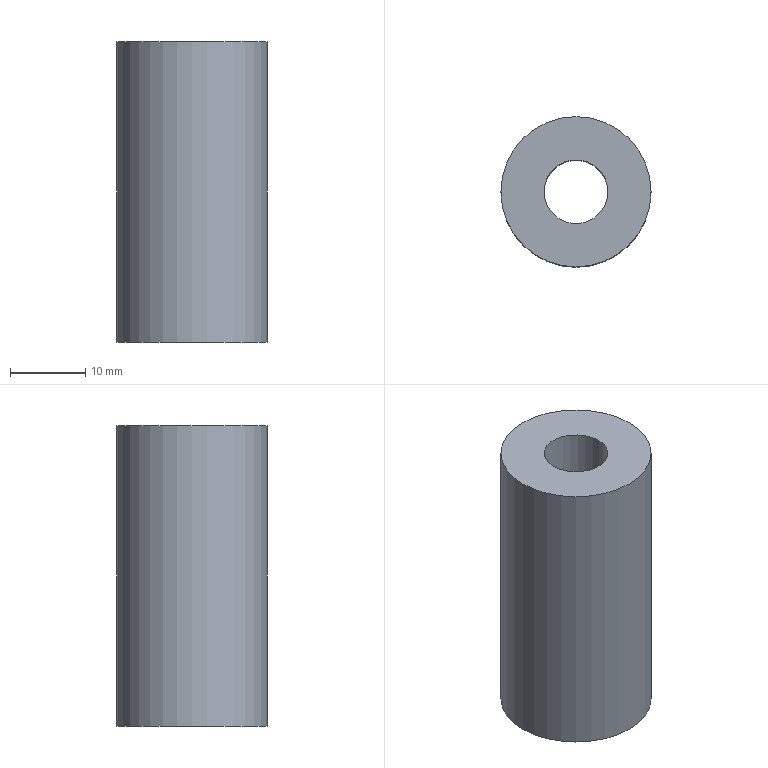Part | STEP file | S2 | 1 solid | 4 faces | box 20 x 20 x 40 mm | volume 10297 mm3 | cylinder 2 | plane 2 | commonest cylinder face diameters 8.5 x1 20 x1
STEP:
#1=CARTESIAN_POINT('',(0.,0.,0.));
#2=DIRECTION('',(0.,0.,1.));
#3=DIRECTION('',(1.,0.,0.));
#4=AXIS2_PLACEMENT_3D('',#1,#2,#3);
#5=CARTESIAN_POINT('',(4.25,0.,40.));
#6=VERTEX_POINT('',#5);
#7=CARTESIAN_POINT('',(0.,0.,40.));
#8=DIRECTION('',(0.,0.,-1.));
#9=DIRECTION('',(-1.,0.,0.));
#10=AXIS2_PLACEMENT_3D('',#7,#8,#9);
#11=CIRCLE('',#10,4.25);
#12=CARTESIAN_POINT('',(0.,0.,0.));
#13=DIRECTION('',(0.,0.,1.));
#14=DIRECTION('',(-1.,0.,0.));
#15=AXIS2_PLACEMENT_3D('',#12,#13,#14);
#16=CYLINDRICAL_SURFACE('',#15,4.25);
#17=CARTESIAN_POINT('',(12.566,40.));
#18=DIRECTION('',(-1.,0.));
#19=VECTOR('',#18,1.);
#20=LINE('',#17,#19);
#21=(GEOMETRIC_REPRESENTATION_CONTEXT(2)PARAMETRIC_REPRESENTATION_CONTEXT()REPRESENTATION_CONTEXT('',''));
#22=DEFINITIONAL_REPRESENTATION('',(#20),#21);
#23=PCURVE('',#16,#22);
#24=CARTESIAN_POINT('',(0.,0.,40.));
#25=DIRECTION('',(0.,0.,1.));
#26=DIRECTION('',(1.,0.,0.));
#27=AXIS2_PLACEMENT_3D('',#24,#25,#26);
#28=PLANE('',#27);
#29=CARTESIAN_POINT('',(-4.25,0.));
#30=CARTESIAN_POINT('',(-4.25,7.361));
#31=CARTESIAN_POINT('',(2.125,3.681));
#32=CARTESIAN_POINT('',(8.5,0.));
#33=CARTESIAN_POINT('',(2.125,-3.681));
#34=CARTESIAN_POINT('',(-4.25,-7.361));
#35=CARTESIAN_POINT('',(-4.25,0.));
#36=(BOUNDED_CURVE()B_SPLINE_CURVE(2,(#29,#30,#31,#32,#33,#34,#35),.UNSPECIFIED.,.T.,.F.)B_SPLINE_CURVE_WITH_KNOTS((1,2,2,2,2,1),(-2.094,0.,2.094,4.189,6.283,8.378),.UNSPECIFIED.)CURVE()GEOMETRIC_REPRESENTATION_ITEM()RATIONAL_B_SPLINE_CURVE((1.,0.5,1.,0.5,1.,0.5,1.))REPRESENTATION_ITEM(''));
#37=(GEOMETRIC_REPRESENTATION_CONTEXT(2)PARAMETRIC_REPRESENTATION_CONTEXT()REPRESENTATION_CONTEXT('',''));
#38=DEFINITIONAL_REPRESENTATION('',(#36),#37);
#39=PCURVE('',#28,#38);
#40=SURFACE_CURVE('',#11,(#23,#39),.PCURVE_S1.);
#41=EDGE_CURVE('',#6,#6,#40,.T.);
#42=ORIENTED_EDGE('',*,*,#41,.T.);
#43=CARTESIAN_POINT('',(4.25,0.,0.));
#44=VERTEX_POINT('',#43);
#45=CARTESIAN_POINT('',(4.25,0.,0.));
#46=CARTESIAN_POINT('',(4.25,0.,40.));
#47=B_SPLINE_CURVE_WITH_KNOTS('',1,(#45,#46),.UNSPECIFIED.,.F.,.F.,(2,2),(0.,40.),.PIECEWISE_BEZIER_KNOTS.);
#48=CARTESIAN_POINT('',(3.142,0.));
#49=DIRECTION('',(0.,1.));
#50=VECTOR('',#49,1.);
#51=LINE('',#48,#50);
#52=(GEOMETRIC_REPRESENTATION_CONTEXT(2)PARAMETRIC_REPRESENTATION_CONTEXT()REPRESENTATION_CONTEXT('',''));
#53=DEFINITIONAL_REPRESENTATION('',(#51),#52);
#54=PCURVE('',#16,#53);
#55=CARTESIAN_POINT('',(9.425,0.));
#56=DIRECTION('',(0.,1.));
#57=VECTOR('',#56,1.);
#58=LINE('',#55,#57);
#59=(GEOMETRIC_REPRESENTATION_CONTEXT(2)PARAMETRIC_REPRESENTATION_CONTEXT()REPRESENTATION_CONTEXT('',''));
#60=DEFINITIONAL_REPRESENTATION('',(#58),#59);
#61=PCURVE('',#16,#60);
#62=SEAM_CURVE('',#47,(#54,#61),.PCURVE_S1.);
#63=EDGE_CURVE('',#44,#6,#62,.T.);
#64=ORIENTED_EDGE('',*,*,#63,.F.);
#65=CARTESIAN_POINT('',(0.,0.,0.));
#66=DIRECTION('',(0.,0.,1.));
#67=DIRECTION('',(-1.,0.,0.));
#68=AXIS2_PLACEMENT_3D('',#65,#66,#67);
#69=CIRCLE('',#68,4.25);
#70=CARTESIAN_POINT('',(0.,0.));
#71=DIRECTION('',(1.,0.));
#72=VECTOR('',#71,1.);
#73=LINE('',#70,#72);
#74=(GEOMETRIC_REPRESENTATION_CONTEXT(2)PARAMETRIC_REPRESENTATION_CONTEXT()REPRESENTATION_CONTEXT('',''));
#75=DEFINITIONAL_REPRESENTATION('',(#73),#74);
#76=PCURVE('',#16,#75);
#77=CARTESIAN_POINT('',(0.,0.,0.));
#78=DIRECTION('',(0.,0.,1.));
#79=DIRECTION('',(1.,0.,0.));
#80=AXIS2_PLACEMENT_3D('',#77,#78,#79);
#81=PLANE('',#80);
#82=CARTESIAN_POINT('',(0.,0.));
#83=DIRECTION('',(-1.,0.));
#84=AXIS2_PLACEMENT_2D('',#82,#83);
#85=CIRCLE('',#84,4.25);
#86=(GEOMETRIC_REPRESENTATION_CONTEXT(2)PARAMETRIC_REPRESENTATION_CONTEXT()REPRESENTATION_CONTEXT('',''));
#87=DEFINITIONAL_REPRESENTATION('',(#85),#86);
#88=PCURVE('',#81,#87);
#89=SURFACE_CURVE('',#69,(#76,#88),.PCURVE_S1.);
#90=EDGE_CURVE('',#44,#44,#89,.T.);
#91=ORIENTED_EDGE('',*,*,#90,.T.);
#92=ORIENTED_EDGE('',*,*,#63,.T.);
#93=EDGE_LOOP('',(#42,#64,#91,#92));
#94=FACE_BOUND('',#93,.F.);
#95=ADVANCED_FACE('',(#94),#16,.F.);
#96=CARTESIAN_POINT('',(10.,0.,40.));
#97=VERTEX_POINT('',#96);
#98=CARTESIAN_POINT('',(0.,0.,40.));
#99=DIRECTION('',(0.,0.,1.));
#100=DIRECTION('',(-1.,0.,0.));
#101=AXIS2_PLACEMENT_3D('',#98,#99,#100);
#102=CIRCLE('',#101,10.);
#103=CARTESIAN_POINT('',(0.,0.,0.));
#104=DIRECTION('',(0.,0.,1.));
#105=DIRECTION('',(-1.,0.,0.));
#106=AXIS2_PLACEMENT_3D('',#103,#104,#105);
#107=CYLINDRICAL_SURFACE('',#106,10.);
#108=CARTESIAN_POINT('',(0.,40.));
#109=DIRECTION('',(1.,0.));
#110=VECTOR('',#109,1.);
#111=LINE('',#108,#110);
#112=(GEOMETRIC_REPRESENTATION_CONTEXT(2)PARAMETRIC_REPRESENTATION_CONTEXT()REPRESENTATION_CONTEXT('',''));
#113=DEFINITIONAL_REPRESENTATION('',(#111),#112);
#114=PCURVE('',#107,#113);
#115=CARTESIAN_POINT('',(0.,0.));
#116=DIRECTION('',(-1.,0.));
#117=AXIS2_PLACEMENT_2D('',#115,#116);
#118=CIRCLE('',#117,10.);
#119=(GEOMETRIC_REPRESENTATION_CONTEXT(2)PARAMETRIC_REPRESENTATION_CONTEXT()REPRESENTATION_CONTEXT('',''));
#120=DEFINITIONAL_REPRESENTATION('',(#118),#119);
#121=PCURVE('',#28,#120);
#122=SURFACE_CURVE('',#102,(#114,#121),.PCURVE_S1.);
#123=EDGE_CURVE('',#97,#97,#122,.T.);
#124=ORIENTED_EDGE('',*,*,#123,.F.);
#125=CARTESIAN_POINT('',(10.,0.,0.));
#126=VERTEX_POINT('',#125);
#127=CARTESIAN_POINT('',(10.,0.,0.));
#128=CARTESIAN_POINT('',(10.,0.,40.));
#129=B_SPLINE_CURVE_WITH_KNOTS('',1,(#127,#128),.UNSPECIFIED.,.F.,.F.,(2,2),(0.,40.),.PIECEWISE_BEZIER_KNOTS.);
#130=CARTESIAN_POINT('',(3.142,0.));
#131=DIRECTION('',(0.,1.));
#132=VECTOR('',#131,1.);
#133=LINE('',#130,#132);
#134=(GEOMETRIC_REPRESENTATION_CONTEXT(2)PARAMETRIC_REPRESENTATION_CONTEXT()REPRESENTATION_CONTEXT('',''));
#135=DEFINITIONAL_REPRESENTATION('',(#133),#134);
#136=PCURVE('',#107,#135);
#137=CARTESIAN_POINT('',(9.425,0.));
#138=DIRECTION('',(0.,1.));
#139=VECTOR('',#138,1.);
#140=LINE('',#137,#139);
#141=(GEOMETRIC_REPRESENTATION_CONTEXT(2)PARAMETRIC_REPRESENTATION_CONTEXT()REPRESENTATION_CONTEXT('',''));
#142=DEFINITIONAL_REPRESENTATION('',(#140),#141);
#143=PCURVE('',#107,#142);
#144=SEAM_CURVE('',#129,(#136,#143),.PCURVE_S1.);
#145=EDGE_CURVE('',#126,#97,#144,.T.);
#146=ORIENTED_EDGE('',*,*,#145,.F.);
#147=CARTESIAN_POINT('',(0.,0.,0.));
#148=DIRECTION('',(0.,0.,-1.));
#149=DIRECTION('',(-1.,0.,0.));
#150=AXIS2_PLACEMENT_3D('',#147,#148,#149);
#151=CIRCLE('',#150,10.);
#152=CARTESIAN_POINT('',(12.566,0.));
#153=DIRECTION('',(-1.,0.));
#154=VECTOR('',#153,1.);
#155=LINE('',#152,#154);
#156=(GEOMETRIC_REPRESENTATION_CONTEXT(2)PARAMETRIC_REPRESENTATION_CONTEXT()REPRESENTATION_CONTEXT('',''));
#157=DEFINITIONAL_REPRESENTATION('',(#155),#156);
#158=PCURVE('',#107,#157);
#159=CARTESIAN_POINT('',(-10.,0.));
#160=CARTESIAN_POINT('',(-10.,17.321));
#161=CARTESIAN_POINT('',(5.,8.66));
#162=CARTESIAN_POINT('',(20.,0.));
#163=CARTESIAN_POINT('',(5.,-8.66));
#164=CARTESIAN_POINT('',(-10.,-17.321));
#165=CARTESIAN_POINT('',(-10.,0.));
#166=(BOUNDED_CURVE()B_SPLINE_CURVE(2,(#159,#160,#161,#162,#163,#164,#165),.UNSPECIFIED.,.T.,.F.)B_SPLINE_CURVE_WITH_KNOTS((1,2,2,2,2,1),(-2.094,0.,2.094,4.189,6.283,8.378),.UNSPECIFIED.)CURVE()GEOMETRIC_REPRESENTATION_ITEM()RATIONAL_B_SPLINE_CURVE((1.,0.5,1.,0.5,1.,0.5,1.))REPRESENTATION_ITEM(''));
#167=(GEOMETRIC_REPRESENTATION_CONTEXT(2)PARAMETRIC_REPRESENTATION_CONTEXT()REPRESENTATION_CONTEXT('',''));
#168=DEFINITIONAL_REPRESENTATION('',(#166),#167);
#169=PCURVE('',#81,#168);
#170=SURFACE_CURVE('',#151,(#158,#169),.PCURVE_S1.);
#171=EDGE_CURVE('',#126,#126,#170,.T.);
#172=ORIENTED_EDGE('',*,*,#171,.F.);
#173=ORIENTED_EDGE('',*,*,#145,.T.);
#174=EDGE_LOOP('',(#124,#146,#172,#173));
#175=FACE_BOUND('',#174,.T.);
#176=ADVANCED_FACE('',(#175),#107,.T.);
#177=ORIENTED_EDGE('',*,*,#171,.T.);
#178=EDGE_LOOP('',(#177));
#179=FACE_BOUND('',#178,.T.);
#180=ORIENTED_EDGE('',*,*,#90,.T.);
#181=EDGE_LOOP('',(#180));
#182=FACE_BOUND('',#181,.T.);
#183=ADVANCED_FACE('',(#179,#182),#81,.F.);
#184=ORIENTED_EDGE('',*,*,#123,.T.);
#185=EDGE_LOOP('',(#184));
#186=FACE_BOUND('',#185,.T.);
#187=ORIENTED_EDGE('',*,*,#41,.T.);
#188=EDGE_LOOP('',(#187));
#189=FACE_BOUND('',#188,.T.);
#190=ADVANCED_FACE('',(#186,#189),#28,.T.);
#191=CLOSED_SHELL('',(#95,#176,#183,#190));
#192=MANIFOLD_SOLID_BREP('',#191);
#193=(LENGTH_UNIT()NAMED_UNIT(*)SI_UNIT(.MILLI.,.METRE.));
#194=UNCERTAINTY_MEASURE_WITH_UNIT(LENGTH_MEASURE(0.00001),#193,'','');
#195=(NAMED_UNIT(*)PLANE_ANGLE_UNIT()SI_UNIT($,.RADIAN.));
#196=(NAMED_UNIT(*)SI_UNIT($,.STERADIAN.)SOLID_ANGLE_UNIT());
#197=(GEOMETRIC_REPRESENTATION_CONTEXT(3)GLOBAL_UNCERTAINTY_ASSIGNED_CONTEXT((#194))GLOBAL_UNIT_ASSIGNED_CONTEXT((#193,#195,#196))REPRESENTATION_CONTEXT('',''));
#198=ADVANCED_BREP_SHAPE_REPRESENTATION('',(#4,#192),#197);